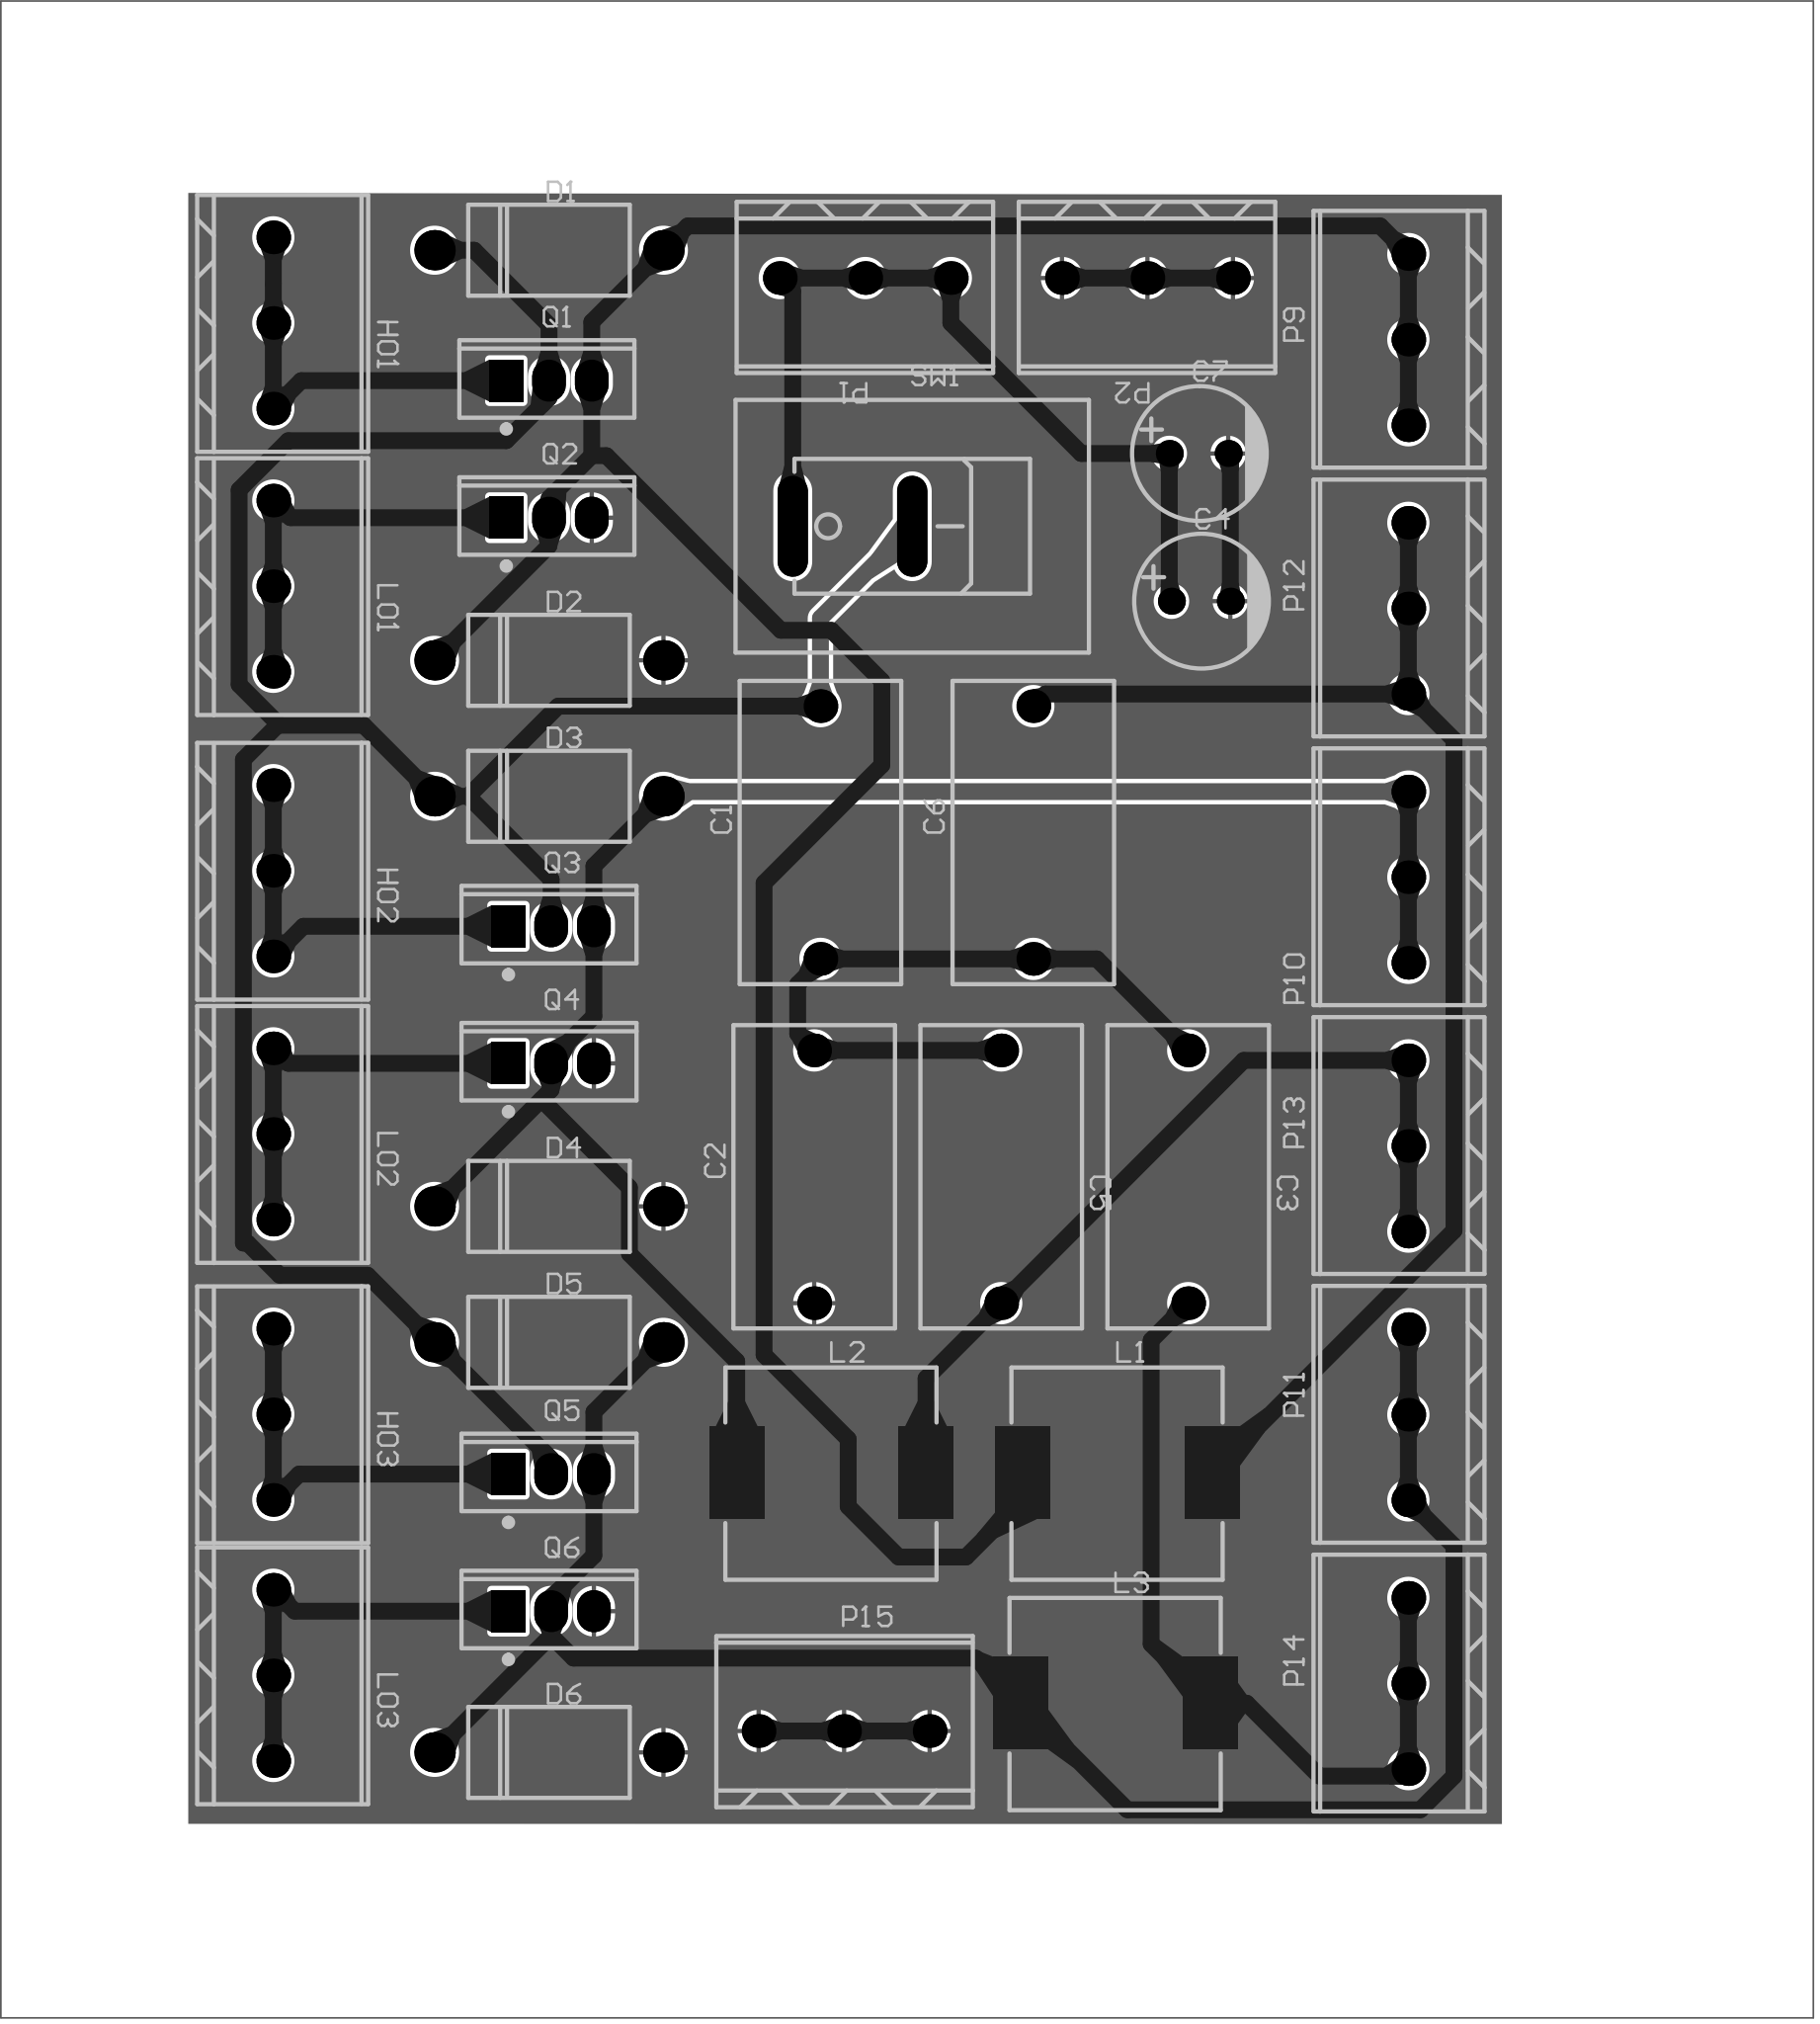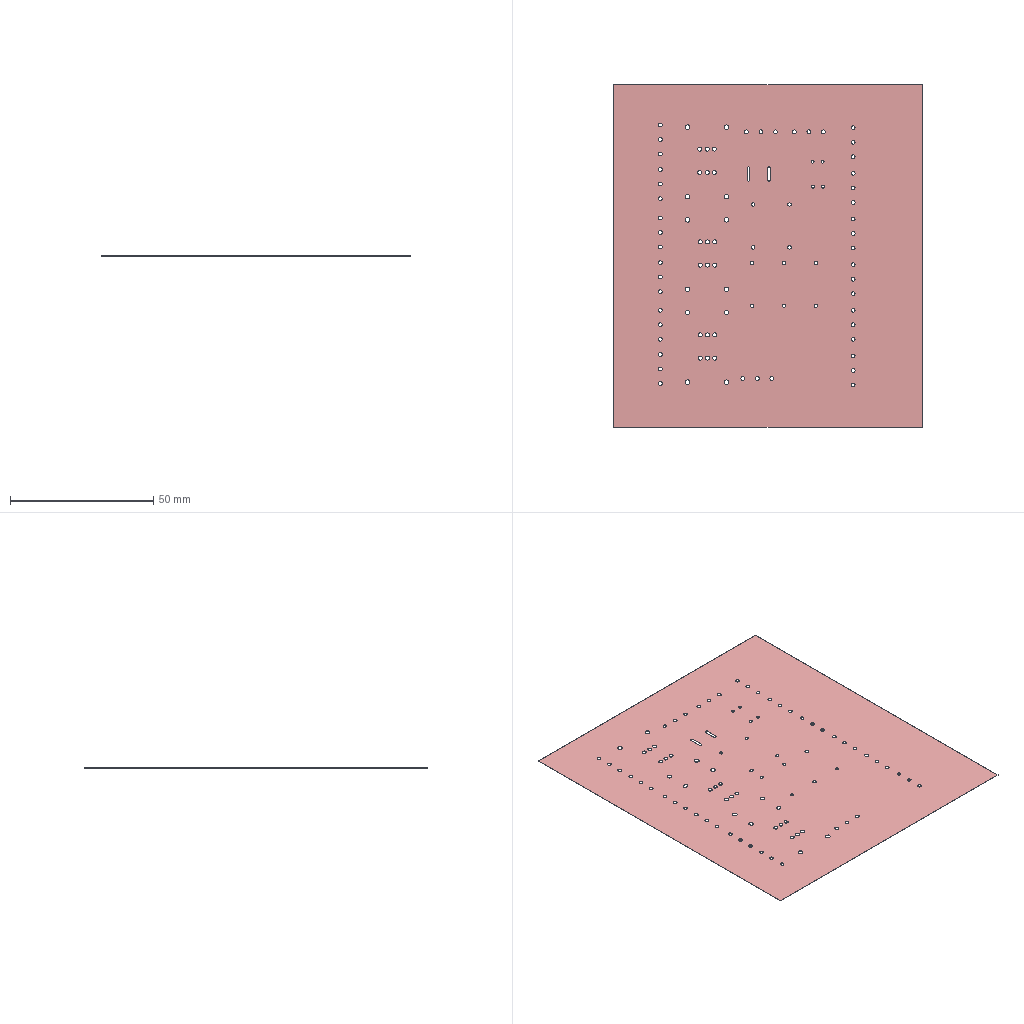Circuit board layout | Altium Designer | box 107.7 x 119.7 x 0.1 mm
Layer stack:
# Altium Designer layer stack of  (unit mm; dielectric type: 0 none, 1 core, 2 prepreg, 3 surface material)
index,name,kind,layer,copper_thickness_mm,dielectric_type,dielectric_thickness_mm,dielectric_material,dielectric_constant
0,Top Paste Mask Layer,other,,,,,,
1,Top Silkscreen Layer,other,,,,,,
2,Top Solder Mask Layer,dielectric,,,3,0.01,,3.3
3,Top Layer,copper,Top Layer,0.035,,,,
4,Bottom Layer,copper,Bottom Layer,0.035,,,,
5,Bottom Solder Mask Layer,dielectric,,,3,0.01,,3.3
6,Bottom Silkscreen Layer,other,,,,,,
7,Bottom Paste Mask Layer,other,,,,,,
# drill layer pairs: low layer,high layer
drill_pair,Top Layer,Bottom Layer
Part placement:
Designator,Comment,Layer,Footprint,Center-X(mm),Center-Y(mm),Rotation
P1,DC supply V1 positive,TopLayer,CONN-TH_3P-P5.00_WJ500V-5.08-3P,121.219,173.108,180
P2,DC supply V1 negative,TopLayer,CONN-TH_3P-P5.00_WJ500V-5.08-3P,137.982,173.108,180
HO1,First channel high-level control input,TopLayer,CONN-TH_3P-P5.00_WJ500V-5.08-3P,86.04,170.441,270
LO1,First channel low-level control input,TopLayer,CONN-TH_3P-P5.00_WJ500V-5.08-3P,86.04,154.82,270
HO2,Second channel high-level control input,TopLayer,CONN-TH_3P-P5.00_WJ500V-5.08-3P,86.04,137.929,270
LO2,Second channel low-level control input,TopLayer,CONN-TH_3P-P5.00_WJ500V-5.08-3P,86.04,122.308,270
HO3,Third channel high-level control input,TopLayer,CONN-TH_3P-P5.00_WJ500V-5.08-3P,86.04,105.671,270
LO3,Third channel low-level control input,TopLayer,CONN-TH_3P-P5.00_WJ500V-5.08-3P,86.04,90.177,270
P9,Provides first channel reference voltage,TopLayer,CONN-TH_3P-P5.00_WJ500V-5.08-3P,153.486,169.45,90
P10,Provides second channel reference voltage,TopLayer,CONN-TH_3P-P5.00_WJ500V-5.08-3P,153.486,137.548,90
P11,Provides third channel reference voltage,TopLayer,CONN-TH_3P-P5.00_WJ500V-5.08-3P,153.486,105.646,90
P12,First channel load,TopLayer,CONN-TH_3P-P5.00_WJ500V-5.08-3P,153.486,153.499,90
P13,Second channel load,TopLayer,CONN-TH_3P-P5.00_WJ500V-5.08-3P,153.486,121.597,90
P14,Third channel load,TopLayer,CONN-TH_3P-P5.00_WJ500V-5.08-3P,153.486,89.694,90
P15,Add ground interface,TopLayer,CONN-TH_3P-P5.00_WJ500V-5.08-3P,119.958,86.875,0
C1,1uF,TopLayer,CAP-TH_L18.0-W9.5-P15.00-D1.2,118.552,140.2,90
C2,1uF,TopLayer,CAP-TH_L18.0-W9.5-P15.00-D1.2,118.18,119.768,90
C3,1uF,TopLayer,CAP-TH_L18.0-W9.5-P15.00-D1.2,140.405,119.768,270
C5,1uF,TopLayer,CAP-TH_L18.0-W9.5-P15.00-D1.2,129.292,119.768,270
C6,1uF,TopLayer,CAP-TH_L18.0-W9.5-P15.00-D1.2,131.2,140.2,90
Q1,IRF540N,TopLayer,TO-220AB-3_L10.4-W4.6-P2.54-L,102.422,167.019,0
Q2,IRF540N,TopLayer,TO-220AB-3_L10.4-W4.6-P2.54-L,102.422,158.884,0
Q3,IRF540N,TopLayer,TO-220AB-3_L10.4-W4.6-P2.54-L,102.549,134.634,0
Q4,IRF540N,TopLayer,TO-220AB-3_L10.4-W4.6-P2.54-L,102.549,126.499,0
Q5,IRF540N,TopLayer,TO-220AB-3_L10.4-W4.6-P2.54-L,102.549,102.122,0
Q6,IRF540N,TopLayer,TO-220AB-3_L10.4-W4.6-P2.54-L,102.549,93.987,0
C7,100uF, voltage stabilising,TopLayer,CAP-TH_BD8.0-P3.50-D1.0-FD,141.03,162.694,0
D1,FR307,TopLayer,DO-201AD_BD5.3-L8.4-P12.50-D1.4-RD,102.422,174.759,0
D2,FR307,TopLayer,DO-201AD_BD5.3-L8.4-P12.50-D1.4-RD,102.422,150.42,0
D3,FR307,TopLayer,DO-201AD_BD5.3-L8.4-P12.50-D1.4-RD,102.422,142.352,0
D4,FR307,TopLayer,DO-201AD_BD5.3-L8.4-P12.50-D1.4-RD,102.422,118.013,0
D5,FR307,TopLayer,DO-201AD_BD5.3-L8.4-P12.50-D1.4-RD,102.422,109.944,0
D6,FR307,TopLayer,DO-201AD_BD5.3-L8.4-P12.50-D1.4-RD,102.422,85.605,0
L1,100uH,TopLayer,IND-SMD_L13.5-W12.6_125CDMCC-DS,136.2,102.2,0
L2,100uH,TopLayer,IND-SMD_L13.5-W12.6_125CDMCC-DS,119.2,102.2,0
L3,100uH,TopLayer,IND-SMD_L13.5-W12.6_125CDMCC-DS,136.087,88.526,0
SW1,MR1-110-C5N-BB,TopLayer,SW-TH_MR1-110-C5N-BB,120.456,158.376,0
C4,100uF, voltage stabilising,TopLayer,CAP-TH_BD8.0-P3.50-D1.0-FD,141.157,153.931,0
Pad and via stacks:
# Altium Designer via and pad stacks of  (unit mm). Each distinct definition once, with the count of objects using it.
# via: kind,start_layer,end_layer,hole_mm,diameter_mm,mode(0 simple;1 top-mid-bottom;2 full stack),diameter_per_layer,count,example_net
# pad: kind,layer,hole_mm,hole_type(0 round;1 square;2 slot),plating,top_size,top_shape(1 round;2 rect;3 octagon;9 rounded rect),mid_size,bottom_size,mode,footprint,size_per_layer,count,example
pad,Multi-Layer,1.3,0,plated,2x2,1,2x2,2x2,0,CONN-TH_3P-P5.00_WJ500V-5.08-3P,,45,P1.3
pad,Multi-Layer,1.2,0,plated,2x2,1,2x2,2x2,0,CAP-TH_L18.0-W9.5-P15.00-D1.2,,10,C1.1
pad,Multi-Layer,1.4,0,plated,2x2.5,1,2x2.5,2x2.5,0,TO-220AB-3_L10.4-W4.6-P2.54-L,,12,Q1.2
pad,Multi-Layer,1.4,0,plated,2x2.5,2,2x2.5,2x2.5,0,TO-220AB-3_L10.4-W4.6-P2.54-L,,6,Q1.1
pad,Multi-Layer,1,0,plated,1.6x1.6,1,1.6x1.6,1.6x1.6,0,CAP-TH_BD8.0-P3.50-D1.0-FD,,4,C7.2
pad,Multi-Layer,1.6,0,plated,2.4x2.4,1,2.4x2.4,2.4x2.4,0,DO-201AD_BD5.3-L8.4-P12.50-D1.4-RD,,12,D1.2
pad,Multi-Layer,1,2,plated,1.8x6,1,1.8x6,1.8x6,0,SW-TH_MR1-110-C5N-BB,,2,SW1.1
pad,Top Layer,0,0,plated,3.25x5.5,2,3.25x5.5,3.25x5.5,0,IND-SMD_L13.5-W12.6_125CDMCC-DS,,6,L1.1
Copper pours:
name,layer,net,type(0 solid;1 hatched;2 none)
Bottom Layer-GND,Bottom Layer,GND,0
Design rules, without the lines most boards share:
# Altium Designer design rules of  (exported by Altium Designer, unit mm)
# columns: name | kind | enabled | priority | scope1 | scope2 | descriptor | typed fields (field=value)
Default | 0 | enabled | 1 | All | All | Clearance Constraint (Gap=6mil) (All),(All) | gap=0.1524
Default_1 | 63 | enabled | 1 | All | All | Board Clearance Constraint (Gap=0mil) (All) |
otherClearance | 52 | enabled | 1 | All | All | Hole To Hole Clearance (Gap=11.8mil) (All),(All) | gap=0.2997
Default_2 | 2 | enabled | 1 | All | All | Width Constraint (Min=10mil) (Max=1000mil) (Preferred=10mil) (All) |
differentialPair | 51 | enabled | 1 | All | All | Differential Pairs Uncoupled Length using the Gap Constraints (Min=5mil) (Max=6mil) (Prefered=6mil)  and Width Constraints (Min=5mil) (Max=100mil) (Prefered=100mil) (All) |
Default_3 | 11 | enabled | 1 | All | All | Routing Via (MinHoleWidth=12.008mil) (MaxHoleWidth=1181mil) (PreferredHoleWidth=12.008mil) (MinWidth=24.016mil) (MaxWidth=1969mil) (PreferedWidth=24.016mil) (All) | via_min_hole=0.305 via_max_hole=29.997 via_preferred_diameter=0.61 via_preferred_hole=0.305
Common | 13 | enabled | 2 | All | All | Solder Mask Expansion (Expansion =2mil) (All) | expansion=0.0508
Common_1 | 13 | enabled | 1 | IsVia | All | Solder Mask Expansion (Expansion =-1000mil) (IsVia) | expansion=-25.4